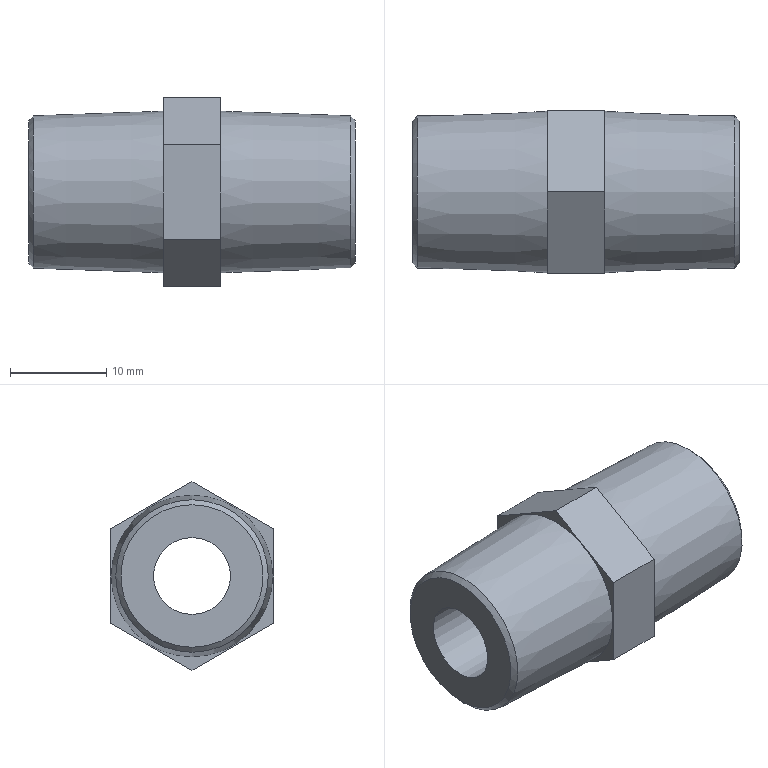Part | STEP file | solid 133 | 1 solid | 15 faces | box 34 x 17 x 19.63 mm | volume 5633 mm3 | plane 10 | cone 4 | cylinder 1 | commonest cylinder face diameters 8 x1